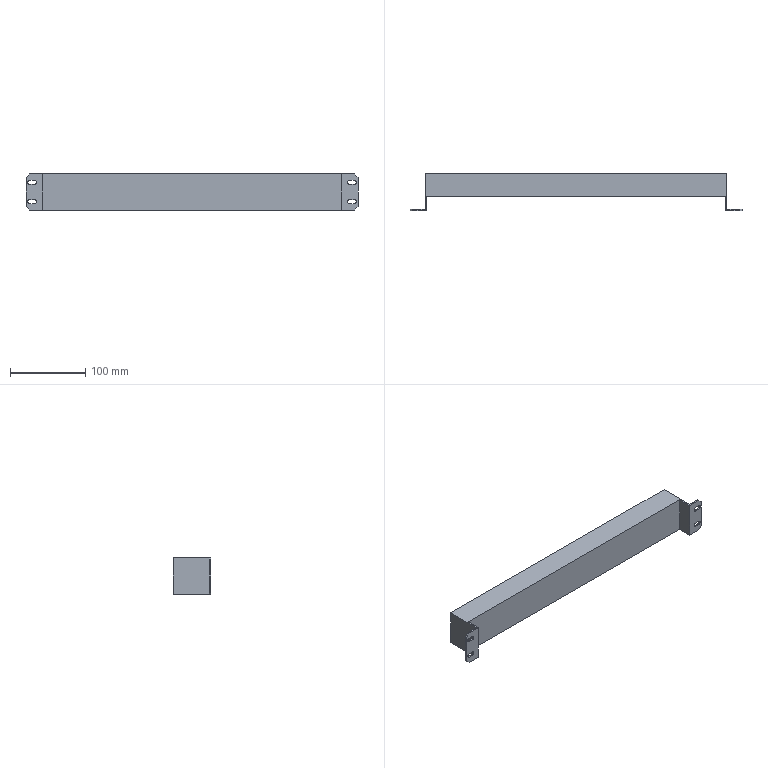Part | SolidWorks | features BaseBody 1 | 1 solid | 34 faces | box 440 x 50 x 48 mm | volume 602134 mm3 | plane 26 | cylinder 8 | commonest cylinder face diameters 5.5 x8
STEP:
#1=CARTESIAN_POINT('',(215.,-17.,15.5));
#2=VERTEX_POINT('',#1);
#3=CARTESIAN_POINT('',(215.,-17.,10.));
#4=VERTEX_POINT('',#3);
#5=CARTESIAN_POINT('',(215.,-17.,12.75));
#6=DIRECTION('',(0.,1.,0.));
#7=DIRECTION('',(0.,0.,1.));
#8=AXIS2_PLACEMENT_3D('',#5,#6,#7);
#9=CIRCLE('',#8,2.75);
#10=EDGE_CURVE('',#2,#4,#9,.T.);
#11=ORIENTED_EDGE('',*,*,#10,.T.);
#12=CARTESIAN_POINT('',(215.,-19.,10.));
#13=VERTEX_POINT('',#12);
#14=CARTESIAN_POINT('',(215.,-37.,10.));
#15=DIRECTION('',(0.,-1.,0.));
#16=VECTOR('',#15,1000.);
#17=LINE('',#14,#16);
#18=EDGE_CURVE('',#4,#13,#17,.T.);
#19=ORIENTED_EDGE('',*,*,#18,.T.);
#20=CARTESIAN_POINT('',(215.,-19.,15.5));
#21=VERTEX_POINT('',#20);
#22=CARTESIAN_POINT('',(215.,-19.,12.75));
#23=DIRECTION('',(0.,-1.,0.));
#24=DIRECTION('',(0.,0.,1.));
#25=AXIS2_PLACEMENT_3D('',#22,#23,#24);
#26=CIRCLE('',#25,2.75);
#27=EDGE_CURVE('',#13,#21,#26,.T.);
#28=ORIENTED_EDGE('',*,*,#27,.T.);
#29=CARTESIAN_POINT('',(215.,-37.,15.5));
#30=DIRECTION('',(0.,1.,0.));
#31=VECTOR('',#30,1000.);
#32=LINE('',#29,#31);
#33=EDGE_CURVE('',#21,#2,#32,.T.);
#34=ORIENTED_EDGE('',*,*,#33,.T.);
#35=EDGE_LOOP('',(#11,#19,#28,#34));
#36=FACE_OUTER_BOUND('',#35,.T.);
#37=CARTESIAN_POINT('',(215.,-37.,12.75));
#38=DIRECTION('',(0.,1.,0.));
#39=DIRECTION('',(0.,0.,1.));
#40=AXIS2_PLACEMENT_3D('',#37,#38,#39);
#41=CYLINDRICAL_SURFACE('',#40,2.75);
#42=ADVANCED_FACE('',(#36),#41,.F.);
#43=CARTESIAN_POINT('',(209.,-17.,15.5));
#44=VERTEX_POINT('',#43);
#45=CARTESIAN_POINT('',(220.,-17.,15.5));
#46=DIRECTION('',(1.,0.,0.));
#47=VECTOR('',#46,1000.);
#48=LINE('',#45,#47);
#49=EDGE_CURVE('',#44,#2,#48,.T.);
#50=ORIENTED_EDGE('',*,*,#49,.T.);
#51=ORIENTED_EDGE('',*,*,#33,.F.);
#52=CARTESIAN_POINT('',(209.,-19.,15.5));
#53=VERTEX_POINT('',#52);
#54=CARTESIAN_POINT('',(0.,-19.,15.5));
#55=DIRECTION('',(-1.,0.,0.));
#56=VECTOR('',#55,1000.);
#57=LINE('',#54,#56);
#58=EDGE_CURVE('',#21,#53,#57,.T.);
#59=ORIENTED_EDGE('',*,*,#58,.T.);
#60=CARTESIAN_POINT('',(209.,-37.,15.5));
#61=DIRECTION('',(0.,1.,0.));
#62=VECTOR('',#61,1000.);
#63=LINE('',#60,#62);
#64=EDGE_CURVE('',#53,#44,#63,.T.);
#65=ORIENTED_EDGE('',*,*,#64,.T.);
#66=EDGE_LOOP('',(#50,#51,#59,#65));
#67=FACE_OUTER_BOUND('',#66,.T.);
#68=CARTESIAN_POINT('',(209.,-37.,15.5));
#69=DIRECTION('',(0.,0.,1.));
#70=DIRECTION('',(0.,-1.,0.));
#71=AXIS2_PLACEMENT_3D('',#68,#69,#70);
#72=PLANE('',#71);
#73=ADVANCED_FACE('',(#67),#72,.F.);
#74=CARTESIAN_POINT('',(209.,-17.,10.));
#75=VERTEX_POINT('',#74);
#76=CARTESIAN_POINT('',(209.,-17.,12.75));
#77=DIRECTION('',(0.,1.,0.));
#78=DIRECTION('',(0.,0.,1.));
#79=AXIS2_PLACEMENT_3D('',#76,#77,#78);
#80=CIRCLE('',#79,2.75);
#81=EDGE_CURVE('',#75,#44,#80,.T.);
#82=ORIENTED_EDGE('',*,*,#81,.T.);
#83=ORIENTED_EDGE('',*,*,#64,.F.);
#84=CARTESIAN_POINT('',(209.,-19.,10.));
#85=VERTEX_POINT('',#84);
#86=CARTESIAN_POINT('',(209.,-19.,12.75));
#87=DIRECTION('',(0.,-1.,0.));
#88=DIRECTION('',(0.,0.,1.));
#89=AXIS2_PLACEMENT_3D('',#86,#87,#88);
#90=CIRCLE('',#89,2.75);
#91=EDGE_CURVE('',#53,#85,#90,.T.);
#92=ORIENTED_EDGE('',*,*,#91,.T.);
#93=CARTESIAN_POINT('',(209.,-37.,10.));
#94=DIRECTION('',(0.,1.,0.));
#95=VECTOR('',#94,1000.);
#96=LINE('',#93,#95);
#97=EDGE_CURVE('',#85,#75,#96,.T.);
#98=ORIENTED_EDGE('',*,*,#97,.T.);
#99=EDGE_LOOP('',(#82,#83,#92,#98));
#100=FACE_OUTER_BOUND('',#99,.T.);
#101=CARTESIAN_POINT('',(209.,-37.,12.75));
#102=DIRECTION('',(0.,1.,0.));
#103=DIRECTION('',(0.,0.,1.));
#104=AXIS2_PLACEMENT_3D('',#101,#102,#103);
#105=CYLINDRICAL_SURFACE('',#104,2.75);
#106=ADVANCED_FACE('',(#100),#105,.F.);
#107=CARTESIAN_POINT('',(220.,-17.,10.));
#108=DIRECTION('',(-1.,0.,0.));
#109=VECTOR('',#108,1000.);
#110=LINE('',#107,#109);
#111=EDGE_CURVE('',#4,#75,#110,.T.);
#112=ORIENTED_EDGE('',*,*,#111,.T.);
#113=ORIENTED_EDGE('',*,*,#97,.F.);
#114=CARTESIAN_POINT('',(0.,-19.,10.));
#115=DIRECTION('',(1.,0.,0.));
#116=VECTOR('',#115,1000.);
#117=LINE('',#114,#116);
#118=EDGE_CURVE('',#85,#13,#117,.T.);
#119=ORIENTED_EDGE('',*,*,#118,.T.);
#120=ORIENTED_EDGE('',*,*,#18,.F.);
#121=EDGE_LOOP('',(#112,#113,#119,#120));
#122=FACE_OUTER_BOUND('',#121,.T.);
#123=CARTESIAN_POINT('',(209.,-37.,10.));
#124=DIRECTION('',(0.,0.,-1.));
#125=DIRECTION('',(-1.,0.,0.));
#126=AXIS2_PLACEMENT_3D('',#123,#124,#125);
#127=PLANE('',#126);
#128=ADVANCED_FACE('',(#122),#127,.F.);
#129=CARTESIAN_POINT('',(215.,-17.,-10.));
#130=VERTEX_POINT('',#129);
#131=CARTESIAN_POINT('',(215.,-17.,-15.5));
#132=VERTEX_POINT('',#131);
#133=CARTESIAN_POINT('',(215.,-17.,-12.75));
#134=DIRECTION('',(0.,1.,0.));
#135=DIRECTION('',(0.,0.,1.));
#136=AXIS2_PLACEMENT_3D('',#133,#134,#135);
#137=CIRCLE('',#136,2.75);
#138=EDGE_CURVE('',#130,#132,#137,.T.);
#139=ORIENTED_EDGE('',*,*,#138,.T.);
#140=CARTESIAN_POINT('',(215.,-19.,-15.5));
#141=VERTEX_POINT('',#140);
#142=CARTESIAN_POINT('',(215.,-37.,-15.5));
#143=DIRECTION('',(0.,-1.,0.));
#144=VECTOR('',#143,1000.);
#145=LINE('',#142,#144);
#146=EDGE_CURVE('',#132,#141,#145,.T.);
#147=ORIENTED_EDGE('',*,*,#146,.T.);
#148=CARTESIAN_POINT('',(215.,-19.,-10.));
#149=VERTEX_POINT('',#148);
#150=CARTESIAN_POINT('',(215.,-19.,-12.75));
#151=DIRECTION('',(0.,-1.,0.));
#152=DIRECTION('',(0.,0.,1.));
#153=AXIS2_PLACEMENT_3D('',#150,#151,#152);
#154=CIRCLE('',#153,2.75);
#155=EDGE_CURVE('',#141,#149,#154,.T.);
#156=ORIENTED_EDGE('',*,*,#155,.T.);
#157=CARTESIAN_POINT('',(215.,-37.,-10.));
#158=DIRECTION('',(0.,1.,0.));
#159=VECTOR('',#158,1000.);
#160=LINE('',#157,#159);
#161=EDGE_CURVE('',#149,#130,#160,.T.);
#162=ORIENTED_EDGE('',*,*,#161,.T.);
#163=EDGE_LOOP('',(#139,#147,#156,#162));
#164=FACE_OUTER_BOUND('',#163,.T.);
#165=CARTESIAN_POINT('',(215.,-37.,-12.75));
#166=DIRECTION('',(0.,1.,0.));
#167=DIRECTION('',(0.,0.,1.));
#168=AXIS2_PLACEMENT_3D('',#165,#166,#167);
#169=CYLINDRICAL_SURFACE('',#168,2.75);
#170=ADVANCED_FACE('',(#164),#169,.F.);
#171=CARTESIAN_POINT('',(209.,-17.,-10.));
#172=VERTEX_POINT('',#171);
#173=CARTESIAN_POINT('',(220.,-17.,-10.));
#174=DIRECTION('',(1.,0.,0.));
#175=VECTOR('',#174,1000.);
#176=LINE('',#173,#175);
#177=EDGE_CURVE('',#172,#130,#176,.T.);
#178=ORIENTED_EDGE('',*,*,#177,.T.);
#179=ORIENTED_EDGE('',*,*,#161,.F.);
#180=CARTESIAN_POINT('',(209.,-19.,-10.));
#181=VERTEX_POINT('',#180);
#182=CARTESIAN_POINT('',(0.,-19.,-10.));
#183=DIRECTION('',(-1.,0.,0.));
#184=VECTOR('',#183,1000.);
#185=LINE('',#182,#184);
#186=EDGE_CURVE('',#149,#181,#185,.T.);
#187=ORIENTED_EDGE('',*,*,#186,.T.);
#188=CARTESIAN_POINT('',(209.,-37.,-10.));
#189=DIRECTION('',(0.,1.,0.));
#190=VECTOR('',#189,1000.);
#191=LINE('',#188,#190);
#192=EDGE_CURVE('',#181,#172,#191,.T.);
#193=ORIENTED_EDGE('',*,*,#192,.T.);
#194=EDGE_LOOP('',(#178,#179,#187,#193));
#195=FACE_OUTER_BOUND('',#194,.T.);
#196=CARTESIAN_POINT('',(209.,-37.,-10.));
#197=DIRECTION('',(0.,0.,1.));
#198=DIRECTION('',(0.,-1.,0.));
#199=AXIS2_PLACEMENT_3D('',#196,#197,#198);
#200=PLANE('',#199);
#201=ADVANCED_FACE('',(#195),#200,.F.);
#202=CARTESIAN_POINT('',(209.,-17.,-15.5));
#203=VERTEX_POINT('',#202);
#204=CARTESIAN_POINT('',(209.,-17.,-12.75));
#205=DIRECTION('',(0.,1.,0.));
#206=DIRECTION('',(0.,0.,1.));
#207=AXIS2_PLACEMENT_3D('',#204,#205,#206);
#208=CIRCLE('',#207,2.75);
#209=EDGE_CURVE('',#203,#172,#208,.T.);
#210=ORIENTED_EDGE('',*,*,#209,.T.);
#211=ORIENTED_EDGE('',*,*,#192,.F.);
#212=CARTESIAN_POINT('',(209.,-19.,-15.5));
#213=VERTEX_POINT('',#212);
#214=CARTESIAN_POINT('',(209.,-19.,-12.75));
#215=DIRECTION('',(0.,-1.,0.));
#216=DIRECTION('',(0.,0.,1.));
#217=AXIS2_PLACEMENT_3D('',#214,#215,#216);
#218=CIRCLE('',#217,2.75);
#219=EDGE_CURVE('',#181,#213,#218,.T.);
#220=ORIENTED_EDGE('',*,*,#219,.T.);
#221=CARTESIAN_POINT('',(209.,-37.,-15.5));
#222=DIRECTION('',(0.,1.,0.));
#223=VECTOR('',#222,1000.);
#224=LINE('',#221,#223);
#225=EDGE_CURVE('',#213,#203,#224,.T.);
#226=ORIENTED_EDGE('',*,*,#225,.T.);
#227=EDGE_LOOP('',(#210,#211,#220,#226));
#228=FACE_OUTER_BOUND('',#227,.T.);
#229=CARTESIAN_POINT('',(209.,-37.,-12.75));
#230=DIRECTION('',(0.,1.,0.));
#231=DIRECTION('',(0.,0.,1.));
#232=AXIS2_PLACEMENT_3D('',#229,#230,#231);
#233=CYLINDRICAL_SURFACE('',#232,2.75);
#234=ADVANCED_FACE('',(#228),#233,.F.);
#235=CARTESIAN_POINT('',(220.,-17.,-15.5));
#236=DIRECTION('',(-1.,0.,0.));
#237=VECTOR('',#236,1000.);
#238=LINE('',#235,#237);
#239=EDGE_CURVE('',#132,#203,#238,.T.);
#240=ORIENTED_EDGE('',*,*,#239,.T.);
#241=ORIENTED_EDGE('',*,*,#225,.F.);
#242=CARTESIAN_POINT('',(0.,-19.,-15.5));
#243=DIRECTION('',(1.,0.,0.));
#244=VECTOR('',#243,1000.);
#245=LINE('',#242,#244);
#246=EDGE_CURVE('',#213,#141,#245,.T.);
#247=ORIENTED_EDGE('',*,*,#246,.T.);
#248=ORIENTED_EDGE('',*,*,#146,.F.);
#249=EDGE_LOOP('',(#240,#241,#247,#248));
#250=FACE_OUTER_BOUND('',#249,.T.);
#251=CARTESIAN_POINT('',(209.,-37.,-15.5));
#252=DIRECTION('',(0.,0.,-1.));
#253=DIRECTION('',(-1.,0.,0.));
#254=AXIS2_PLACEMENT_3D('',#251,#252,#253);
#255=PLANE('',#254);
#256=ADVANCED_FACE('',(#250),#255,.F.);
#257=CARTESIAN_POINT('',(220.,-17.,-19.));
#258=VERTEX_POINT('',#257);
#259=CARTESIAN_POINT('',(220.,-17.,19.));
#260=VERTEX_POINT('',#259);
#261=CARTESIAN_POINT('',(220.,-17.,-24.));
#262=DIRECTION('',(0.,0.,1.));
#263=VECTOR('',#262,1000.);
#264=LINE('',#261,#263);
#265=EDGE_CURVE('',#258,#260,#264,.T.);
#266=ORIENTED_EDGE('',*,*,#265,.T.);
#267=CARTESIAN_POINT('',(220.,-19.,19.));
#268=VERTEX_POINT('',#267);
#269=CARTESIAN_POINT('',(220.,0.,19.));
#270=DIRECTION('',(0.,1.,0.));
#271=VECTOR('',#270,1000.);
#272=LINE('',#269,#271);
#273=EDGE_CURVE('',#268,#260,#272,.T.);
#274=ORIENTED_EDGE('',*,*,#273,.F.);
#275=CARTESIAN_POINT('',(220.,-19.,-19.));
#276=VERTEX_POINT('',#275);
#277=CARTESIAN_POINT('',(220.,-19.,0.));
#278=DIRECTION('',(0.,0.,-1.));
#279=VECTOR('',#278,1000.);
#280=LINE('',#277,#279);
#281=EDGE_CURVE('',#268,#276,#280,.T.);
#282=ORIENTED_EDGE('',*,*,#281,.T.);
#283=CARTESIAN_POINT('',(220.,0.,-19.));
#284=DIRECTION('',(0.,-1.,0.));
#285=VECTOR('',#284,1000.);
#286=LINE('',#283,#285);
#287=EDGE_CURVE('',#258,#276,#286,.T.);
#288=ORIENTED_EDGE('',*,*,#287,.F.);
#289=EDGE_LOOP('',(#266,#274,#282,#288));
#290=FACE_OUTER_BOUND('',#289,.T.);
#291=CARTESIAN_POINT('',(220.,0.,0.));
#292=DIRECTION('',(1.,0.,0.));
#293=DIRECTION('',(0.,1.,0.));
#294=AXIS2_PLACEMENT_3D('',#291,#292,#293);
#295=PLANE('',#294);
#296=ADVANCED_FACE('',(#290),#295,.T.);
#297=CARTESIAN_POINT('',(-209.,-17.,-15.5));
#298=VERTEX_POINT('',#297);
#299=CARTESIAN_POINT('',(-209.,-17.,-10.));
#300=VERTEX_POINT('',#299);
#301=CARTESIAN_POINT('',(-209.,-17.,-12.75));
#302=DIRECTION('',(0.,-1.,0.));
#303=DIRECTION('',(0.,0.,1.));
#304=AXIS2_PLACEMENT_3D('',#301,#302,#303);
#305=CIRCLE('',#304,2.75);
#306=EDGE_CURVE('',#298,#300,#305,.T.);
#307=ORIENTED_EDGE('',*,*,#306,.F.);
#308=CARTESIAN_POINT('',(-209.,-19.,-15.5));
#309=VERTEX_POINT('',#308);
#310=CARTESIAN_POINT('',(-209.,-37.,-15.5));
#311=DIRECTION('',(0.,-1.,0.));
#312=VECTOR('',#311,1000.);
#313=LINE('',#310,#312);
#314=EDGE_CURVE('',#298,#309,#313,.T.);
#315=ORIENTED_EDGE('',*,*,#314,.T.);
#316=CARTESIAN_POINT('',(-209.,-19.,-10.));
#317=VERTEX_POINT('',#316);
#318=CARTESIAN_POINT('',(-209.,-19.,-12.75));
#319=DIRECTION('',(0.,-1.,0.));
#320=DIRECTION('',(0.,0.,1.));
#321=AXIS2_PLACEMENT_3D('',#318,#319,#320);
#322=CIRCLE('',#321,2.75);
#323=EDGE_CURVE('',#309,#317,#322,.T.);
#324=ORIENTED_EDGE('',*,*,#323,.T.);
#325=CARTESIAN_POINT('',(-209.,-37.,-10.));
#326=DIRECTION('',(0.,1.,0.));
#327=VECTOR('',#326,1000.);
#328=LINE('',#325,#327);
#329=EDGE_CURVE('',#317,#300,#328,.T.);
#330=ORIENTED_EDGE('',*,*,#329,.T.);
#331=EDGE_LOOP('',(#307,#315,#324,#330));
#332=FACE_OUTER_BOUND('',#331,.T.);
#333=CARTESIAN_POINT('',(-209.,-37.,-12.75));
#334=DIRECTION('',(0.,1.,0.));
#335=DIRECTION('',(0.,0.,1.));
#336=AXIS2_PLACEMENT_3D('',#333,#334,#335);
#337=CYLINDRICAL_SURFACE('',#336,2.75);
#338=ADVANCED_FACE('',(#332),#337,.F.);
#339=CARTESIAN_POINT('',(-215.,-17.,-10.));
#340=VERTEX_POINT('',#339);
#341=CARTESIAN_POINT('',(-220.,-17.,-10.));
#342=DIRECTION('',(-1.,0.,0.));
#343=VECTOR('',#342,1000.);
#344=LINE('',#341,#343);
#345=EDGE_CURVE('',#300,#340,#344,.T.);
#346=ORIENTED_EDGE('',*,*,#345,.F.);
#347=ORIENTED_EDGE('',*,*,#329,.F.);
#348=CARTESIAN_POINT('',(-215.,-19.,-10.));
#349=VERTEX_POINT('',#348);
#350=CARTESIAN_POINT('',(0.,-19.,-10.));
#351=DIRECTION('',(-1.,0.,0.));
#352=VECTOR('',#351,1000.);
#353=LINE('',#350,#352);
#354=EDGE_CURVE('',#317,#349,#353,.T.);
#355=ORIENTED_EDGE('',*,*,#354,.T.);
#356=CARTESIAN_POINT('',(-215.,-37.,-10.));
#357=DIRECTION('',(0.,1.,0.));
#358=VECTOR('',#357,1000.);
#359=LINE('',#356,#358);
#360=EDGE_CURVE('',#349,#340,#359,.T.);
#361=ORIENTED_EDGE('',*,*,#360,.T.);
#362=EDGE_LOOP('',(#346,#347,#355,#361));
#363=FACE_OUTER_BOUND('',#362,.T.);
#364=CARTESIAN_POINT('',(-209.,-37.,-10.));
#365=DIRECTION('',(0.,0.,1.));
#366=DIRECTION('',(0.,-1.,0.));
#367=AXIS2_PLACEMENT_3D('',#364,#365,#366);
#368=PLANE('',#367);
#369=ADVANCED_FACE('',(#363),#368,.F.);
#370=CARTESIAN_POINT('',(-215.,-17.,-15.5));
#371=VERTEX_POINT('',#370);
#372=CARTESIAN_POINT('',(-215.,-17.,-12.75));
#373=DIRECTION('',(0.,-1.,0.));
#374=DIRECTION('',(0.,0.,1.));
#375=AXIS2_PLACEMENT_3D('',#372,#373,#374);
#376=CIRCLE('',#375,2.75);
#377=EDGE_CURVE('',#340,#371,#376,.T.);
#378=ORIENTED_EDGE('',*,*,#377,.F.);
#379=ORIENTED_EDGE('',*,*,#360,.F.);
#380=CARTESIAN_POINT('',(-215.,-19.,-15.5));
#381=VERTEX_POINT('',#380);
#382=CARTESIAN_POINT('',(-215.,-19.,-12.75));
#383=DIRECTION('',(0.,-1.,0.));
#384=DIRECTION('',(0.,0.,1.));
#385=AXIS2_PLACEMENT_3D('',#382,#383,#384);
#386=CIRCLE('',#385,2.75);
#387=EDGE_CURVE('',#349,#381,#386,.T.);
#388=ORIENTED_EDGE('',*,*,#387,.T.);
#389=CARTESIAN_POINT('',(-215.,-37.,-15.5));
#390=DIRECTION('',(0.,1.,0.));
#391=VECTOR('',#390,1000.);
#392=LINE('',#389,#391);
#393=EDGE_CURVE('',#381,#371,#392,.T.);
#394=ORIENTED_EDGE('',*,*,#393,.T.);
#395=EDGE_LOOP('',(#378,#379,#388,#394));
#396=FACE_OUTER_BOUND('',#395,.T.);
#397=CARTESIAN_POINT('',(-215.,-37.,-12.75));
#398=DIRECTION('',(0.,1.,0.));
#399=DIRECTION('',(0.,0.,1.));
#400=AXIS2_PLACEMENT_3D('',#397,#398,#399);
#401=CYLINDRICAL_SURFACE('',#400,2.75);
#402=ADVANCED_FACE('',(#396),#401,.F.);
#403=CARTESIAN_POINT('',(-220.,-17.,-15.5));
#404=DIRECTION('',(1.,0.,0.));
#405=VECTOR('',#404,1000.);
#406=LINE('',#403,#405);
#407=EDGE_CURVE('',#371,#298,#406,.T.);
#408=ORIENTED_EDGE('',*,*,#407,.F.);
#409=ORIENTED_EDGE('',*,*,#393,.F.);
#410=CARTESIAN_POINT('',(0.,-19.,-15.5));
#411=DIRECTION('',(1.,0.,0.));
#412=VECTOR('',#411,1000.);
#413=LINE('',#410,#412);
#414=EDGE_CURVE('',#381,#309,#413,.T.);
#415=ORIENTED_EDGE('',*,*,#414,.T.);
#416=ORIENTED_EDGE('',*,*,#314,.F.);
#417=EDGE_LOOP('',(#408,#409,#415,#416));
#418=FACE_OUTER_BOUND('',#417,.T.);
#419=CARTESIAN_POINT('',(-209.,-37.,-15.5));
#420=DIRECTION('',(0.,0.,-1.));
#421=DIRECTION('',(0.,-1.,0.));
#422=AXIS2_PLACEMENT_3D('',#419,#420,#421);
#423=PLANE('',#422);
#424=ADVANCED_FACE('',(#418),#423,.F.);
#425=CARTESIAN_POINT('',(-209.,-17.,10.));
#426=VERTEX_POINT('',#425);
#427=CARTESIAN_POINT('',(-209.,-17.,15.5));
#428=VERTEX_POINT('',#427);
#429=CARTESIAN_POINT('',(-209.,-17.,12.75));
#430=DIRECTION('',(0.,-1.,0.));
#431=DIRECTION('',(0.,0.,1.));
#432=AXIS2_PLACEMENT_3D('',#429,#430,#431);
#433=CIRCLE('',#432,2.75);
#434=EDGE_CURVE('',#426,#428,#433,.T.);
#435=ORIENTED_EDGE('',*,*,#434,.F.);
#436=CARTESIAN_POINT('',(-209.,-19.,10.));
#437=VERTEX_POINT('',#436);
#438=CARTESIAN_POINT('',(-209.,-37.,10.));
#439=DIRECTION('',(0.,-1.,0.));
#440=VECTOR('',#439,1000.);
#441=LINE('',#438,#440);
#442=EDGE_CURVE('',#426,#437,#441,.T.);
#443=ORIENTED_EDGE('',*,*,#442,.T.);
#444=CARTESIAN_POINT('',(-209.,-19.,15.5));
#445=VERTEX_POINT('',#444);
#446=CARTESIAN_POINT('',(-209.,-19.,12.75));
#447=DIRECTION('',(0.,-1.,0.));
#448=DIRECTION('',(0.,0.,1.));
#449=AXIS2_PLACEMENT_3D('',#446,#447,#448);
#450=CIRCLE('',#449,2.75);
#451=EDGE_CURVE('',#437,#445,#450,.T.);
#452=ORIENTED_EDGE('',*,*,#451,.T.);
#453=CARTESIAN_POINT('',(-209.,-37.,15.5));
#454=DIRECTION('',(0.,1.,0.));
#455=VECTOR('',#454,1000.);
#456=LINE('',#453,#455);
#457=EDGE_CURVE('',#445,#428,#456,.T.);
#458=ORIENTED_EDGE('',*,*,#457,.T.);
#459=EDGE_LOOP('',(#435,#443,#452,#458));
#460=FACE_OUTER_BOUND('',#459,.T.);
#461=CARTESIAN_POINT('',(-209.,-37.,12.75));
#462=DIRECTION('',(0.,1.,0.));
#463=DIRECTION('',(0.,0.,1.));
#464=AXIS2_PLACEMENT_3D('',#461,#462,#463);
#465=CYLINDRICAL_SURFACE('',#464,2.75);
#466=ADVANCED_FACE('',(#460),#465,.F.);
#467=CARTESIAN_POINT('',(-215.,-17.,15.5));
#468=VERTEX_POINT('',#467);
#469=CARTESIAN_POINT('',(-220.,-17.,15.5));
#470=DIRECTION('',(-1.,0.,0.));
#471=VECTOR('',#470,1000.);
#472=LINE('',#469,#471);
#473=EDGE_CURVE('',#428,#468,#472,.T.);
#474=ORIENTED_EDGE('',*,*,#473,.F.);
#475=ORIENTED_EDGE('',*,*,#457,.F.);
#476=CARTESIAN_POINT('',(-215.,-19.,15.5));
#477=VERTEX_POINT('',#476);
#478=CARTESIAN_POINT('',(0.,-19.,15.5));
#479=DIRECTION('',(-1.,0.,0.));
#480=VECTOR('',#479,1000.);
#481=LINE('',#478,#480);
#482=EDGE_CURVE('',#445,#477,#481,.T.);
#483=ORIENTED_EDGE('',*,*,#482,.T.);
#484=CARTESIAN_POINT('',(-215.,-37.,15.5));
#485=DIRECTION('',(0.,1.,0.));
#486=VECTOR('',#485,1000.);
#487=LINE('',#484,#486);
#488=EDGE_CURVE('',#477,#468,#487,.T.);
#489=ORIENTED_EDGE('',*,*,#488,.T.);
#490=EDGE_LOOP('',(#474,#475,#483,#489));
#491=FACE_OUTER_BOUND('',#490,.T.);
#492=CARTESIAN_POINT('',(-209.,-37.,15.5));
#493=DIRECTION('',(0.,0.,1.));
#494=DIRECTION('',(1.,0.,0.));
#495=AXIS2_PLACEMENT_3D('',#492,#493,#494);
#496=PLANE('',#495);
#497=ADVANCED_FACE('',(#491),#496,.F.);
#498=CARTESIAN_POINT('',(-215.,-17.,10.));
#499=VERTEX_POINT('',#498);
#500=CARTESIAN_POINT('',(-215.,-17.,12.75));
#501=DIRECTION('',(0.,-1.,0.));
#502=DIRECTION('',(0.,0.,1.));
#503=AXIS2_PLACEMENT_3D('',#500,#501,#502);
#504=CIRCLE('',#503,2.75);
#505=EDGE_CURVE('',#468,#499,#504,.T.);
#506=ORIENTED_EDGE('',*,*,#505,.F.);
#507=ORIENTED_EDGE('',*,*,#488,.F.);
#508=CARTESIAN_POINT('',(-215.,-19.,10.));
#509=VERTEX_POINT('',#508);
#510=CARTESIAN_POINT('',(-215.,-19.,12.75));
#511=DIRECTION('',(0.,-1.,0.));
#512=DIRECTION('',(0.,0.,1.));
#513=AXIS2_PLACEMENT_3D('',#510,#511,#512);
#514=CIRCLE('',#513,2.75);
#515=EDGE_CURVE('',#477,#509,#514,.T.);
#516=ORIENTED_EDGE('',*,*,#515,.T.);
#517=CARTESIAN_POINT('',(-215.,-37.,10.));
#518=DIRECTION('',(0.,1.,0.));
#519=VECTOR('',#518,1000.);
#520=LINE('',#517,#519);
#521=EDGE_CURVE('',#509,#499,#520,.T.);
#522=ORIENTED_EDGE('',*,*,#521,.T.);
#523=EDGE_LOOP('',(#506,#507,#516,#522));
#524=FACE_OUTER_BOUND('',#523,.T.);
#525=CARTESIAN_POINT('',(-215.,-37.,12.75));
#526=DIRECTION('',(0.,1.,0.));
#527=DIRECTION('',(0.,0.,1.));
#528=AXIS2_PLACEMENT_3D('',#525,#526,#527);
#529=CYLINDRICAL_SURFACE('',#528,2.75);
#530=ADVANCED_FACE('',(#524),#529,.F.);
#531=CARTESIAN_POINT('',(-220.,-17.,10.));
#532=DIRECTION('',(1.,0.,0.));
#533=VECTOR('',#532,1000.);
#534=LINE('',#531,#533);
#535=EDGE_CURVE('',#499,#426,#534,.T.);
#536=ORIENTED_EDGE('',*,*,#535,.F.);
#537=ORIENTED_EDGE('',*,*,#521,.F.);
#538=CARTESIAN_POINT('',(0.,-19.,10.));
#539=DIRECTION('',(1.,0.,0.));
#540=VECTOR('',#539,1000.);
#541=LINE('',#538,#540);
#542=EDGE_CURVE('',#509,#437,#541,.T.);
#543=ORIENTED_EDGE('',*,*,#542,.T.);
#544=ORIENTED_EDGE('',*,*,#442,.F.);
#545=EDGE_LOOP('',(#536,#537,#543,#544));
#546=FACE_OUTER_BOUND('',#545,.T.);
#547=CARTESIAN_POINT('',(-209.,-37.,10.));
#548=DIRECTION('',(0.,0.,-1.));
#549=DIRECTION('',(-1.,0.,0.));
#550=AXIS2_PLACEMENT_3D('',#547,#548,#549);
#551=PLANE('',#550);
#552=ADVANCED_FACE('',(#546),#551,.F.);
#553=CARTESIAN_POINT('',(-220.,-19.,-19.));
#554=VERTEX_POINT('',#553);
#555=CARTESIAN_POINT('',(-220.,-19.,19.));
#556=VERTEX_POINT('',#555);
#557=CARTESIAN_POINT('',(-220.,-19.,0.));
#558=DIRECTION('',(0.,0.,1.));
#559=VECTOR('',#558,1000.);
#560=LINE('',#557,#559);
#561=EDGE_CURVE('',#554,#556,#560,.T.);
#562=ORIENTED_EDGE('',*,*,#561,.T.);
#563=CARTESIAN_POINT('',(-220.,-17.,19.));
#564=VERTEX_POINT('',#563);
#565=CARTESIAN_POINT('',(-220.,31.,19.));
#566=DIRECTION('',(0.,-1.,0.));
#567=VECTOR('',#566,1000.);
#568=LINE('',#565,#567);
#569=EDGE_CURVE('',#564,#556,#568,.T.);
#570=ORIENTED_EDGE('',*,*,#569,.F.);
#571=CARTESIAN_POINT('',(-220.,-17.,-19.));
#572=VERTEX_POINT('',#571);
#573=CARTESIAN_POINT('',(-220.,-17.,-24.));
#574=DIRECTION('',(0.,0.,1.));
#575=VECTOR('',#574,1000.);
#576=LINE('',#573,#575);
#577=EDGE_CURVE('',#572,#564,#576,.T.);
#578=ORIENTED_EDGE('',*,*,#577,.F.);
#579=CARTESIAN_POINT('',(-220.,31.,-19.));
#580=DIRECTION('',(0.,1.,0.));
#581=VECTOR('',#580,1000.);
#582=LINE('',#579,#581);
#583=EDGE_CURVE('',#554,#572,#582,.T.);
#584=ORIENTED_EDGE('',*,*,#583,.F.);
#585=EDGE_LOOP('',(#562,#570,#578,#584));
#586=FACE_OUTER_BOUND('',#585,.T.);
#587=CARTESIAN_POINT('',(-220.,0.,0.));
#588=DIRECTION('',(-1.,0.,0.));
#589=DIRECTION('',(0.,0.,1.));
#590=AXIS2_PLACEMENT_3D('',#587,#588,#589);
#591=PLANE('',#590);
#592=ADVANCED_FACE('',(#586),#591,.T.);
#593=CARTESIAN_POINT('',(215.,-17.,-24.));
#594=VERTEX_POINT('',#593);
#595=CARTESIAN_POINT('',(215.,-17.,-24.));
#596=DIRECTION('',(0.7071,0.,0.7071));
#597=VECTOR('',#596,1000.);
#598=LINE('',#595,#597);
#599=EDGE_CURVE('',#594,#258,#598,.T.);
#600=ORIENTED_EDGE('',*,*,#599,.T.);
#601=ORIENTED_EDGE('',*,*,#287,.T.);
#602=CARTESIAN_POINT('',(215.,-19.,-24.));
#603=VERTEX_POINT('',#602);
#604=CARTESIAN_POINT('',(220.,-19.,-19.));
#605=DIRECTION('',(-0.7071,0.,-0.7071));
#606=VECTOR('',#605,1000.);
#607=LINE('',#604,#606);
#608=EDGE_CURVE('',#276,#603,#607,.T.);
#609=ORIENTED_EDGE('',*,*,#608,.T.);
#610=CARTESIAN_POINT('',(215.,31.,-24.));
#611=DIRECTION('',(0.,1.,0.));
#612=VECTOR('',#611,1000.);
#613=LINE('',#610,#612);
#614=EDGE_CURVE('',#603,#594,#613,.T.);
#615=ORIENTED_EDGE('',*,*,#614,.T.);
#616=EDGE_LOOP('',(#600,#601,#609,#615));
#617=FACE_OUTER_BOUND('',#616,.T.);
#618=CARTESIAN_POINT('',(220.,0.,-19.));
#619=DIRECTION('',(0.7071,0.,-0.7071));
#620=DIRECTION('',(0.,-1.,0.));
#621=AXIS2_PLACEMENT_3D('',#618,#619,#620);
#622=PLANE('',#621);
#623=ADVANCED_FACE('',(#617),#622,.T.);
#624=CARTESIAN_POINT('',(-215.,-17.,-24.));
#625=VERTEX_POINT('',#624);
#626=CARTESIAN_POINT('',(-215.,-17.,-24.));
#627=DIRECTION('',(-0.7071,0.,0.7071));
#628=VECTOR('',#627,1000.);
#629=LINE('',#626,#628);
#630=EDGE_CURVE('',#625,#572,#629,.T.);
#631=ORIENTED_EDGE('',*,*,#630,.F.);
#632=CARTESIAN_POINT('',(-215.,-19.,-24.));
#633=VERTEX_POINT('',#632);
#634=CARTESIAN_POINT('',(-215.,31.,-24.));
#635=DIRECTION('',(0.,-1.,0.));
#636=VECTOR('',#635,1000.);
#637=LINE('',#634,#636);
#638=EDGE_CURVE('',#625,#633,#637,.T.);
#639=ORIENTED_EDGE('',*,*,#638,.T.);
#640=CARTESIAN_POINT('',(-215.,-19.,-24.));
#641=DIRECTION('',(-0.7071,0.,0.7071));
#642=VECTOR('',#641,1000.);
#643=LINE('',#640,#642);
#644=EDGE_CURVE('',#633,#554,#643,.T.);
#645=ORIENTED_EDGE('',*,*,#644,.T.);
#646=ORIENTED_EDGE('',*,*,#583,.T.);
#647=EDGE_LOOP('',(#631,#639,#645,#646));
#648=FACE_OUTER_BOUND('',#647,.T.);
#649=CARTESIAN_POINT('',(-215.,31.,-24.));
#650=DIRECTION('',(-0.7071,0.,-0.7071));
#651=DIRECTION('',(-0.7071,0.,0.7071));
#652=AXIS2_PLACEMENT_3D('',#649,#650,#651);
#653=PLANE('',#652);
#654=ADVANCED_FACE('',(#648),#653,.T.);
#655=ORIENTED_EDGE('',*,*,#81,.F.);
#656=ORIENTED_EDGE('',*,*,#111,.F.);
#657=ORIENTED_EDGE('',*,*,#10,.F.);
#658=ORIENTED_EDGE('',*,*,#49,.F.);
#659=EDGE_LOOP('',(#655,#656,#657,#658));
#660=FACE_BOUND('',#659,.T.);
#661=ORIENTED_EDGE('',*,*,#209,.F.);
#662=ORIENTED_EDGE('',*,*,#239,.F.);
#663=ORIENTED_EDGE('',*,*,#138,.F.);
#664=ORIENTED_EDGE('',*,*,#177,.F.);
#665=EDGE_LOOP('',(#661,#662,#663,#664));
#666=FACE_BOUND('',#665,.T.);
#667=ORIENTED_EDGE('',*,*,#599,.F.);
#668=CARTESIAN_POINT('',(200.,-17.,-24.));
#669=VERTEX_POINT('',#668);
#670=CARTESIAN_POINT('',(-200.,-17.,-24.));
#671=DIRECTION('',(-1.,0.,0.));
#672=VECTOR('',#671,1000.);
#673=LINE('',#670,#672);
#674=EDGE_CURVE('',#594,#669,#673,.T.);
#675=ORIENTED_EDGE('',*,*,#674,.T.);
#676=CARTESIAN_POINT('',(200.,-17.,24.));
#677=VERTEX_POINT('',#676);
#678=CARTESIAN_POINT('',(200.,-17.,-24.));
#679=DIRECTION('',(0.,0.,1.));
#680=VECTOR('',#679,1000.);
#681=LINE('',#678,#680);
#682=EDGE_CURVE('',#669,#677,#681,.T.);
#683=ORIENTED_EDGE('',*,*,#682,.T.);
#684=CARTESIAN_POINT('',(215.,-17.,24.));
#685=VERTEX_POINT('',#684);
#686=CARTESIAN_POINT('',(-200.,-17.,24.));
#687=DIRECTION('',(1.,0.,0.));
#688=VECTOR('',#687,1000.);
#689=LINE('',#686,#688);
#690=EDGE_CURVE('',#677,#685,#689,.T.);
#691=ORIENTED_EDGE('',*,*,#690,.T.);
#692=CARTESIAN_POINT('',(220.,-17.,19.));
#693=DIRECTION('',(-0.7071,0.,0.7071));
#694=VECTOR('',#693,1000.);
#695=LINE('',#692,#694);
#696=EDGE_CURVE('',#260,#685,#695,.T.);
#697=ORIENTED_EDGE('',*,*,#696,.F.);
#698=ORIENTED_EDGE('',*,*,#265,.F.);
#699=EDGE_LOOP('',(#667,#675,#683,#691,#697,#698));
#700=FACE_OUTER_BOUND('',#699,.T.);
#701=CARTESIAN_POINT('',(220.,-17.,-24.));
#702=DIRECTION('',(0.,-1.,0.));
#703=DIRECTION('',(0.,0.,-1.));
#704=AXIS2_PLACEMENT_3D('',#701,#702,#703);
#705=PLANE('',#704);
#706=ADVANCED_FACE('',(#660,#666,#700),#705,.F.);
#707=CARTESIAN_POINT('',(215.,-19.,24.));
#708=VERTEX_POINT('',#707);
#709=CARTESIAN_POINT('',(215.,-19.,24.));
#710=DIRECTION('',(0.7071,0.,-0.7071));
#711=VECTOR('',#710,1000.);
#712=LINE('',#709,#711);
#713=EDGE_CURVE('',#708,#268,#712,.T.);
#714=ORIENTED_EDGE('',*,*,#713,.T.);
#715=ORIENTED_EDGE('',*,*,#273,.T.);
#716=ORIENTED_EDGE('',*,*,#696,.T.);
#717=CARTESIAN_POINT('',(215.,31.,24.));
#718=DIRECTION('',(0.,-1.,0.));
#719=VECTOR('',#718,1000.);
#720=LINE('',#717,#719);
#721=EDGE_CURVE('',#685,#708,#720,.T.);
#722=ORIENTED_EDGE('',*,*,#721,.T.);
#723=EDGE_LOOP('',(#714,#715,#716,#722));
#724=FACE_OUTER_BOUND('',#723,.T.);
#725=CARTESIAN_POINT('',(220.,0.,19.));
#726=DIRECTION('',(0.7071,0.,0.7071));
#727=DIRECTION('',(0.,-1.,0.));
#728=AXIS2_PLACEMENT_3D('',#725,#726,#727);
#729=PLANE('',#728);
#730=ADVANCED_FACE('',(#724),#729,.T.);
#731=ORIENTED_EDGE('',*,*,#91,.F.);
#732=ORIENTED_EDGE('',*,*,#58,.F.);
#733=ORIENTED_EDGE('',*,*,#27,.F.);
#734=ORIENTED_EDGE('',*,*,#118,.F.);
#735=EDGE_LOOP('',(#731,#732,#733,#734));
#736=FACE_BOUND('',#735,.T.);
#737=ORIENTED_EDGE('',*,*,#219,.F.);
#738=ORIENTED_EDGE('',*,*,#186,.F.);
#739=ORIENTED_EDGE('',*,*,#155,.F.);
#740=ORIENTED_EDGE('',*,*,#246,.F.);
#741=EDGE_LOOP('',(#737,#738,#739,#740));
#742=FACE_BOUND('',#741,.T.);
#743=ORIENTED_EDGE('',*,*,#608,.F.);
#744=ORIENTED_EDGE('',*,*,#281,.F.);
#745=ORIENTED_EDGE('',*,*,#713,.F.);
#746=CARTESIAN_POINT('',(198.,-19.,24.));
#747=VERTEX_POINT('',#746);
#748=CARTESIAN_POINT('',(-200.,-19.,24.));
#749=DIRECTION('',(-1.,0.,0.));
#750=VECTOR('',#749,1000.);
#751=LINE('',#748,#750);
#752=EDGE_CURVE('',#708,#747,#751,.T.);
#753=ORIENTED_EDGE('',*,*,#752,.T.);
#754=CARTESIAN_POINT('',(198.,-19.,-24.));
#755=VERTEX_POINT('',#754);
#756=CARTESIAN_POINT('',(198.,-19.,24.));
#757=DIRECTION('',(0.,0.,-1.));
#758=VECTOR('',#757,1000.);
#759=LINE('',#756,#758);
#760=EDGE_CURVE('',#747,#755,#759,.T.);
#761=ORIENTED_EDGE('',*,*,#760,.T.);
#762=CARTESIAN_POINT('',(-200.,-19.,-24.));
#763=DIRECTION('',(1.,0.,0.));
#764=VECTOR('',#763,1000.);
#765=LINE('',#762,#764);
#766=EDGE_CURVE('',#755,#603,#765,.T.);
#767=ORIENTED_EDGE('',*,*,#766,.T.);
#768=EDGE_LOOP('',(#743,#744,#745,#753,#761,#767));
#769=FACE_OUTER_BOUND('',#768,.T.);
#770=CARTESIAN_POINT('',(0.,-19.,0.));
#771=DIRECTION('',(0.,1.,0.));
#772=DIRECTION('',(1.,0.,0.));
#773=AXIS2_PLACEMENT_3D('',#770,#771,#772);
#774=PLANE('',#773);
#775=ADVANCED_FACE('',(#736,#742,#769),#774,.F.);
#776=ORIENTED_EDGE('',*,*,#760,.F.);
#777=CARTESIAN_POINT('',(198.,0.,24.));
#778=VERTEX_POINT('',#777);
#779=CARTESIAN_POINT('',(198.,31.,24.));
#780=DIRECTION('',(0.,1.,0.));
#781=VECTOR('',#780,1000.);
#782=LINE('',#779,#781);
#783=EDGE_CURVE('',#747,#778,#782,.T.);
#784=ORIENTED_EDGE('',*,*,#783,.T.);
#785=CARTESIAN_POINT('',(198.,0.,-24.));
#786=VERTEX_POINT('',#785);
#787=CARTESIAN_POINT('',(198.,0.,0.));
#788=DIRECTION('',(0.,0.,-1.));
#789=VECTOR('',#788,1000.);
#790=LINE('',#787,#789);
#791=EDGE_CURVE('',#778,#786,#790,.T.);
#792=ORIENTED_EDGE('',*,*,#791,.T.);
#793=CARTESIAN_POINT('',(198.,31.,-24.));
#794=DIRECTION('',(0.,-1.,0.));
#795=VECTOR('',#794,1000.);
#796=LINE('',#793,#795);
#797=EDGE_CURVE('',#786,#755,#796,.T.);
#798=ORIENTED_EDGE('',*,*,#797,.T.);
#799=EDGE_LOOP('',(#776,#784,#792,#798));
#800=FACE_OUTER_BOUND('',#799,.T.);
#801=CARTESIAN_POINT('',(198.,-117.042,24.));
#802=DIRECTION('',(1.,0.,0.));
#803=DIRECTION('',(0.,1.,0.));
#804=AXIS2_PLACEMENT_3D('',#801,#802,#803);
#805=PLANE('',#804);
#806=ADVANCED_FACE('',(#800),#805,.F.);
#807=CARTESIAN_POINT('',(-198.,0.,-24.));
#808=VERTEX_POINT('',#807);
#809=CARTESIAN_POINT('',(-198.,0.,24.));
#810=VERTEX_POINT('',#809);
#811=CARTESIAN_POINT('',(-198.,0.,24.));
#812=DIRECTION('',(0.,0.,1.));
#813=VECTOR('',#812,1000.);
#814=LINE('',#811,#813);
#815=EDGE_CURVE('',#808,#810,#814,.T.);
#816=ORIENTED_EDGE('',*,*,#815,.F.);
#817=CARTESIAN_POINT('',(-200.,0.,-24.));
#818=DIRECTION('',(1.,0.,0.));
#819=VECTOR('',#818,1000.);
#820=LINE('',#817,#819);
#821=EDGE_CURVE('',#808,#786,#820,.T.);
#822=ORIENTED_EDGE('',*,*,#821,.T.);
#823=ORIENTED_EDGE('',*,*,#791,.F.);
#824=CARTESIAN_POINT('',(-200.,0.,24.));
#825=DIRECTION('',(-1.,0.,0.));
#826=VECTOR('',#825,1000.);
#827=LINE('',#824,#826);
#828=EDGE_CURVE('',#778,#810,#827,.T.);
#829=ORIENTED_EDGE('',*,*,#828,.T.);
#830=EDGE_LOOP('',(#816,#822,#823,#829));
#831=FACE_OUTER_BOUND('',#830,.T.);
#832=CARTESIAN_POINT('',(0.,0.,0.));
#833=DIRECTION('',(0.,1.,0.));
#834=DIRECTION('',(1.,0.,0.));
#835=AXIS2_PLACEMENT_3D('',#832,#833,#834);
#836=PLANE('',#835);
#837=ADVANCED_FACE('',(#831),#836,.F.);
#838=ORIENTED_EDGE('',*,*,#815,.T.);
#839=CARTESIAN_POINT('',(-198.,-19.,24.));
#840=VERTEX_POINT('',#839);
#841=CARTESIAN_POINT('',(-198.,31.,24.));
#842=DIRECTION('',(0.,-1.,0.));
#843=VECTOR('',#842,1000.);
#844=LINE('',#841,#843);
#845=EDGE_CURVE('',#810,#840,#844,.T.);
#846=ORIENTED_EDGE('',*,*,#845,.T.);
#847=CARTESIAN_POINT('',(-198.,-19.,-24.));
#848=VERTEX_POINT('',#847);
#849=CARTESIAN_POINT('',(-198.,-19.,0.));
#850=DIRECTION('',(0.,0.,-1.));
#851=VECTOR('',#850,1000.);
#852=LINE('',#849,#851);
#853=EDGE_CURVE('',#840,#848,#852,.T.);
#854=ORIENTED_EDGE('',*,*,#853,.T.);
#855=CARTESIAN_POINT('',(-198.,31.,-24.));
#856=DIRECTION('',(0.,1.,0.));
#857=VECTOR('',#856,1000.);
#858=LINE('',#855,#857);
#859=EDGE_CURVE('',#848,#808,#858,.T.);
#860=ORIENTED_EDGE('',*,*,#859,.T.);
#861=EDGE_LOOP('',(#838,#846,#854,#860));
#862=FACE_OUTER_BOUND('',#861,.T.);
#863=CARTESIAN_POINT('',(-198.,-117.042,24.));
#864=DIRECTION('',(1.,0.,0.));
#865=DIRECTION('',(0.,1.,0.));
#866=AXIS2_PLACEMENT_3D('',#863,#864,#865);
#867=PLANE('',#866);
#868=ADVANCED_FACE('',(#862),#867,.T.);
#869=ORIENTED_EDGE('',*,*,#323,.F.);
#870=ORIENTED_EDGE('',*,*,#414,.F.);
#871=ORIENTED_EDGE('',*,*,#387,.F.);
#872=ORIENTED_EDGE('',*,*,#354,.F.);
#873=EDGE_LOOP('',(#869,#870,#871,#872));
#874=FACE_BOUND('',#873,.T.);
#875=ORIENTED_EDGE('',*,*,#451,.F.);
#876=ORIENTED_EDGE('',*,*,#542,.F.);
#877=ORIENTED_EDGE('',*,*,#515,.F.);
#878=ORIENTED_EDGE('',*,*,#482,.F.);
#879=EDGE_LOOP('',(#875,#876,#877,#878));
#880=FACE_BOUND('',#879,.T.);
#881=ORIENTED_EDGE('',*,*,#644,.F.);
#882=CARTESIAN_POINT('',(-200.,-19.,-24.));
#883=DIRECTION('',(1.,0.,0.));
#884=VECTOR('',#883,1000.);
#885=LINE('',#882,#884);
#886=EDGE_CURVE('',#633,#848,#885,.T.);
#887=ORIENTED_EDGE('',*,*,#886,.T.);
#888=ORIENTED_EDGE('',*,*,#853,.F.);
#889=CARTESIAN_POINT('',(-215.,-19.,24.));
#890=VERTEX_POINT('',#889);
#891=CARTESIAN_POINT('',(-200.,-19.,24.));
#892=DIRECTION('',(-1.,0.,0.));
#893=VECTOR('',#892,1000.);
#894=LINE('',#891,#893);
#895=EDGE_CURVE('',#840,#890,#894,.T.);
#896=ORIENTED_EDGE('',*,*,#895,.T.);
#897=CARTESIAN_POINT('',(-215.,-19.,24.));
#898=DIRECTION('',(0.7071,0.,0.7071));
#899=VECTOR('',#898,1000.);
#900=LINE('',#897,#899);
#901=EDGE_CURVE('',#556,#890,#900,.T.);
#902=ORIENTED_EDGE('',*,*,#901,.F.);
#903=ORIENTED_EDGE('',*,*,#561,.F.);
#904=EDGE_LOOP('',(#881,#887,#888,#896,#902,#903));
#905=FACE_OUTER_BOUND('',#904,.T.);
#906=CARTESIAN_POINT('',(0.,-19.,0.));
#907=DIRECTION('',(0.,1.,0.));
#908=DIRECTION('',(1.,0.,0.));
#909=AXIS2_PLACEMENT_3D('',#906,#907,#908);
#910=PLANE('',#909);
#911=ADVANCED_FACE('',(#874,#880,#905),#910,.F.);
#912=ORIENTED_EDGE('',*,*,#901,.T.);
#913=CARTESIAN_POINT('',(-215.,-17.,24.));
#914=VERTEX_POINT('',#913);
#915=CARTESIAN_POINT('',(-215.,31.,24.));
#916=DIRECTION('',(0.,1.,0.));
#917=VECTOR('',#916,1000.);
#918=LINE('',#915,#917);
#919=EDGE_CURVE('',#890,#914,#918,.T.);
#920=ORIENTED_EDGE('',*,*,#919,.T.);
#921=CARTESIAN_POINT('',(-220.,-17.,19.));
#922=DIRECTION('',(0.7071,0.,0.7071));
#923=VECTOR('',#922,1000.);
#924=LINE('',#921,#923);
#925=EDGE_CURVE('',#564,#914,#924,.T.);
#926=ORIENTED_EDGE('',*,*,#925,.F.);
#927=ORIENTED_EDGE('',*,*,#569,.T.);
#928=EDGE_LOOP('',(#912,#920,#926,#927));
#929=FACE_OUTER_BOUND('',#928,.T.);
#930=CARTESIAN_POINT('',(-215.,31.,24.));
#931=DIRECTION('',(-0.7071,0.,0.7071));
#932=DIRECTION('',(0.,1.,0.));
#933=AXIS2_PLACEMENT_3D('',#930,#931,#932);
#934=PLANE('',#933);
#935=ADVANCED_FACE('',(#929),#934,.T.);
#936=ORIENTED_EDGE('',*,*,#377,.T.);
#937=ORIENTED_EDGE('',*,*,#407,.T.);
#938=ORIENTED_EDGE('',*,*,#306,.T.);
#939=ORIENTED_EDGE('',*,*,#345,.T.);
#940=EDGE_LOOP('',(#936,#937,#938,#939));
#941=FACE_BOUND('',#940,.T.);
#942=ORIENTED_EDGE('',*,*,#505,.T.);
#943=ORIENTED_EDGE('',*,*,#535,.T.);
#944=ORIENTED_EDGE('',*,*,#434,.T.);
#945=ORIENTED_EDGE('',*,*,#473,.T.);
#946=EDGE_LOOP('',(#942,#943,#944,#945));
#947=FACE_BOUND('',#946,.T.);
#948=CARTESIAN_POINT('',(-200.,-17.,24.));
#949=VERTEX_POINT('',#948);
#950=CARTESIAN_POINT('',(-200.,-17.,24.));
#951=DIRECTION('',(1.,0.,0.));
#952=VECTOR('',#951,1000.);
#953=LINE('',#950,#952);
#954=EDGE_CURVE('',#914,#949,#953,.T.);
#955=ORIENTED_EDGE('',*,*,#954,.T.);
#956=CARTESIAN_POINT('',(-200.,-17.,-24.));
#957=VERTEX_POINT('',#956);
#958=CARTESIAN_POINT('',(-200.,-17.,-24.));
#959=DIRECTION('',(0.,0.,-1.));
#960=VECTOR('',#959,1000.);
#961=LINE('',#958,#960);
#962=EDGE_CURVE('',#949,#957,#961,.T.);
#963=ORIENTED_EDGE('',*,*,#962,.T.);
#964=CARTESIAN_POINT('',(-200.,-17.,-24.));
#965=DIRECTION('',(-1.,0.,0.));
#966=VECTOR('',#965,1000.);
#967=LINE('',#964,#966);
#968=EDGE_CURVE('',#957,#625,#967,.T.);
#969=ORIENTED_EDGE('',*,*,#968,.T.);
#970=ORIENTED_EDGE('',*,*,#630,.T.);
#971=ORIENTED_EDGE('',*,*,#577,.T.);
#972=ORIENTED_EDGE('',*,*,#925,.T.);
#973=EDGE_LOOP('',(#955,#963,#969,#970,#971,#972));
#974=FACE_OUTER_BOUND('',#973,.T.);
#975=CARTESIAN_POINT('',(-220.,-17.,-24.));
#976=DIRECTION('',(0.,1.,0.));
#977=DIRECTION('',(0.,0.,-1.));
#978=AXIS2_PLACEMENT_3D('',#975,#976,#977);
#979=PLANE('',#978);
#980=ADVANCED_FACE('',(#941,#947,#974),#979,.T.);
#981=CARTESIAN_POINT('',(200.,31.,-24.));
#982=VERTEX_POINT('',#981);
#983=CARTESIAN_POINT('',(200.,31.,-24.));
#984=DIRECTION('',(0.,1.,0.));
#985=VECTOR('',#984,1000.);
#986=LINE('',#983,#985);
#987=EDGE_CURVE('',#669,#982,#986,.T.);
#988=ORIENTED_EDGE('',*,*,#987,.T.);
#989=CARTESIAN_POINT('',(200.,31.,24.));
#990=VERTEX_POINT('',#989);
#991=CARTESIAN_POINT('',(200.,31.,0.));
#992=DIRECTION('',(0.,0.,-1.));
#993=VECTOR('',#992,1000.);
#994=LINE('',#991,#993);
#995=EDGE_CURVE('',#990,#982,#994,.T.);
#996=ORIENTED_EDGE('',*,*,#995,.F.);
#997=CARTESIAN_POINT('',(200.,31.,24.));
#998=DIRECTION('',(0.,-1.,0.));
#999=VECTOR('',#998,1000.);
#1000=LINE('',#997,#999);
#1001=EDGE_CURVE('',#990,#677,#1000,.T.);
#1002=ORIENTED_EDGE('',*,*,#1001,.T.);
#1003=ORIENTED_EDGE('',*,*,#682,.F.);
#1004=EDGE_LOOP('',(#988,#996,#1002,#1003));
#1005=FACE_OUTER_BOUND('',#1004,.T.);
#1006=CARTESIAN_POINT('',(200.,31.,-24.));
#1007=DIRECTION('',(-1.,0.,0.));
#1008=DIRECTION('',(0.,0.,1.));
#1009=AXIS2_PLACEMENT_3D('',#1006,#1007,#1008);
#1010=PLANE('',#1009);
#1011=ADVANCED_FACE('',(#1005),#1010,.F.);
#1012=ORIENTED_EDGE('',*,*,#638,.F.);
#1013=ORIENTED_EDGE('',*,*,#968,.F.);
#1014=CARTESIAN_POINT('',(-200.,31.,-24.));
#1015=VERTEX_POINT('',#1014);
#1016=CARTESIAN_POINT('',(-200.,31.,-24.));
#1017=DIRECTION('',(0.,1.,0.));
#1018=VECTOR('',#1017,1000.);
#1019=LINE('',#1016,#1018);
#1020=EDGE_CURVE('',#957,#1015,#1019,.T.);
#1021=ORIENTED_EDGE('',*,*,#1020,.T.);
#1022=CARTESIAN_POINT('',(0.,31.,-24.));
#1023=DIRECTION('',(-1.,0.,0.));
#1024=VECTOR('',#1023,1000.);
#1025=LINE('',#1022,#1024);
#1026=EDGE_CURVE('',#982,#1015,#1025,.T.);
#1027=ORIENTED_EDGE('',*,*,#1026,.F.);
#1028=ORIENTED_EDGE('',*,*,#987,.F.);
#1029=ORIENTED_EDGE('',*,*,#674,.F.);
#1030=ORIENTED_EDGE('',*,*,#614,.F.);
#1031=ORIENTED_EDGE('',*,*,#766,.F.);
#1032=ORIENTED_EDGE('',*,*,#797,.F.);
#1033=ORIENTED_EDGE('',*,*,#821,.F.);
#1034=ORIENTED_EDGE('',*,*,#859,.F.);
#1035=ORIENTED_EDGE('',*,*,#886,.F.);
#1036=EDGE_LOOP('',(#1012,#1013,#1021,#1027,#1028,#1029,#1030,#1031,#1032,#1033,#1034,#1035));
#1037=FACE_OUTER_BOUND('',#1036,.T.);
#1038=CARTESIAN_POINT('',(-200.,31.,-24.));
#1039=DIRECTION('',(0.,0.,1.));
#1040=DIRECTION('',(1.,0.,0.));
#1041=AXIS2_PLACEMENT_3D('',#1038,#1039,#1040);
#1042=PLANE('',#1041);
#1043=ADVANCED_FACE('',(#1037),#1042,.F.);
#1044=ORIENTED_EDGE('',*,*,#962,.F.);
#1045=CARTESIAN_POINT('',(-200.,31.,24.));
#1046=VERTEX_POINT('',#1045);
#1047=CARTESIAN_POINT('',(-200.,31.,24.));
#1048=DIRECTION('',(0.,1.,0.));
#1049=VECTOR('',#1048,1000.);
#1050=LINE('',#1047,#1049);
#1051=EDGE_CURVE('',#949,#1046,#1050,.T.);
#1052=ORIENTED_EDGE('',*,*,#1051,.T.);
#1053=CARTESIAN_POINT('',(-200.,31.,0.));
#1054=DIRECTION('',(0.,0.,1.));
#1055=VECTOR('',#1054,1000.);
#1056=LINE('',#1053,#1055);
#1057=EDGE_CURVE('',#1015,#1046,#1056,.T.);
#1058=ORIENTED_EDGE('',*,*,#1057,.F.);
#1059=ORIENTED_EDGE('',*,*,#1020,.F.);
#1060=EDGE_LOOP('',(#1044,#1052,#1058,#1059));
#1061=FACE_OUTER_BOUND('',#1060,.T.);
#1062=CARTESIAN_POINT('',(-200.,31.,-24.));
#1063=DIRECTION('',(1.,0.,0.));
#1064=DIRECTION('',(0.,1.,0.));
#1065=AXIS2_PLACEMENT_3D('',#1062,#1063,#1064);
#1066=PLANE('',#1065);
#1067=ADVANCED_FACE('',(#1061),#1066,.F.);
#1068=ORIENTED_EDGE('',*,*,#919,.F.);
#1069=ORIENTED_EDGE('',*,*,#895,.F.);
#1070=ORIENTED_EDGE('',*,*,#845,.F.);
#1071=ORIENTED_EDGE('',*,*,#828,.F.);
#1072=ORIENTED_EDGE('',*,*,#783,.F.);
#1073=ORIENTED_EDGE('',*,*,#752,.F.);
#1074=ORIENTED_EDGE('',*,*,#721,.F.);
#1075=ORIENTED_EDGE('',*,*,#690,.F.);
#1076=ORIENTED_EDGE('',*,*,#1001,.F.);
#1077=CARTESIAN_POINT('',(0.,31.,24.));
#1078=DIRECTION('',(1.,0.,0.));
#1079=VECTOR('',#1078,1000.);
#1080=LINE('',#1077,#1079);
#1081=EDGE_CURVE('',#1046,#990,#1080,.T.);
#1082=ORIENTED_EDGE('',*,*,#1081,.F.);
#1083=ORIENTED_EDGE('',*,*,#1051,.F.);
#1084=ORIENTED_EDGE('',*,*,#954,.F.);
#1085=EDGE_LOOP('',(#1068,#1069,#1070,#1071,#1072,#1073,#1074,#1075,#1076,#1082,#1083,#1084));
#1086=FACE_OUTER_BOUND('',#1085,.T.);
#1087=CARTESIAN_POINT('',(-200.,31.,24.));
#1088=DIRECTION('',(0.,0.,-1.));
#1089=DIRECTION('',(0.,-1.,0.));
#1090=AXIS2_PLACEMENT_3D('',#1087,#1088,#1089);
#1091=PLANE('',#1090);
#1092=ADVANCED_FACE('',(#1086),#1091,.F.);
#1093=ORIENTED_EDGE('',*,*,#1057,.T.);
#1094=ORIENTED_EDGE('',*,*,#1081,.T.);
#1095=ORIENTED_EDGE('',*,*,#995,.T.);
#1096=ORIENTED_EDGE('',*,*,#1026,.T.);
#1097=EDGE_LOOP('',(#1093,#1094,#1095,#1096));
#1098=FACE_OUTER_BOUND('',#1097,.T.);
#1099=CARTESIAN_POINT('',(0.,31.,0.));
#1100=DIRECTION('',(0.,1.,0.));
#1101=DIRECTION('',(1.,0.,0.));
#1102=AXIS2_PLACEMENT_3D('',#1099,#1100,#1101);
#1103=PLANE('',#1102);
#1104=ADVANCED_FACE('',(#1098),#1103,.T.);
#1105=CLOSED_SHELL('',(#42,#73,#106,#128,#170,#201,#234,#256,#296,#338,#369,#402,#424,#466,#497,#530,#552,#592,#623,#654,#706,#730,#775,#806,#837,#868,#911,#935,#980,#1011,#1043,#1067,#1092,#1104));
#1106=MANIFOLD_SOLID_BREP('',#1105);
#1107=CARTESIAN_POINT('',(0.,0.,0.));
#1108=DIRECTION('',(0.,0.,1.));
#1109=DIRECTION('',(1.,0.,0.));
#1110=AXIS2_PLACEMENT_3D('',#1107,#1108,#1109);
#1111=(LENGTH_UNIT()NAMED_UNIT(*)SI_UNIT(.MILLI.,.METRE.));
#1112=UNCERTAINTY_MEASURE_WITH_UNIT(LENGTH_MEASURE(0.00001),#1111,'','');
#1113=(NAMED_UNIT(*)PLANE_ANGLE_UNIT()SI_UNIT($,.RADIAN.));
#1114=(NAMED_UNIT(*)SI_UNIT($,.STERADIAN.)SOLID_ANGLE_UNIT());
#1115=(GEOMETRIC_REPRESENTATION_CONTEXT(3)GLOBAL_UNCERTAINTY_ASSIGNED_CONTEXT((#1112))GLOBAL_UNIT_ASSIGNED_CONTEXT((#1111,#1113,#1114))REPRESENTATION_CONTEXT('',''));
#1116=ADVANCED_BREP_SHAPE_REPRESENTATION('',(#1106,#1110),#1115);